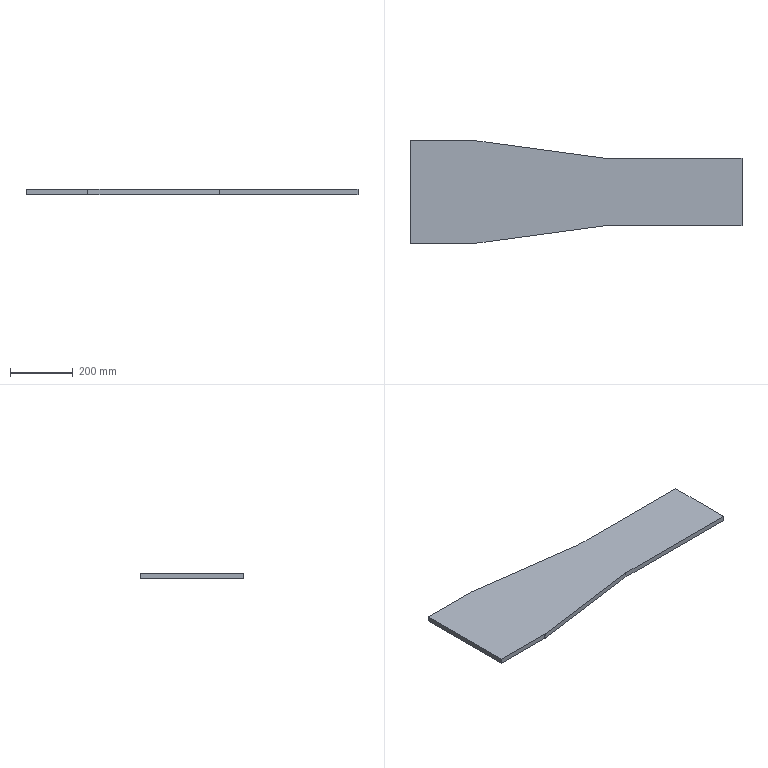Part | SolidWorks | features Extrusion 1 | 1 solid | 12 faces | box 1056 x 330 x 16 mm | volume 4392263 mm3 | plane 10 | cylinder 2 | commonest cylinder face diameters 32 x2
STEP:
#1=CARTESIAN_POINT('',(1056.5,108.,0.));
#2=VERTEX_POINT('',#1);
#3=CARTESIAN_POINT('',(616.5,108.,0.));
#4=VERTEX_POINT('',#3);
#5=CARTESIAN_POINT('',(1056.5,108.,0.));
#6=DIRECTION('',(-1.,0.,0.));
#7=VECTOR('',#6,1000.);
#8=LINE('',#5,#7);
#9=EDGE_CURVE('',#2,#4,#8,.T.);
#10=ORIENTED_EDGE('',*,*,#9,.T.);
#11=CARTESIAN_POINT('',(616.5,108.,16.));
#12=VERTEX_POINT('',#11);
#13=CARTESIAN_POINT('',(616.5,108.,16.));
#14=DIRECTION('',(0.,0.,-1.));
#15=VECTOR('',#14,1000.);
#16=LINE('',#13,#15);
#17=EDGE_CURVE('',#12,#4,#16,.T.);
#18=ORIENTED_EDGE('',*,*,#17,.F.);
#19=CARTESIAN_POINT('',(1056.5,108.,16.));
#20=VERTEX_POINT('',#19);
#21=CARTESIAN_POINT('',(1056.5,108.,16.));
#22=DIRECTION('',(-1.,0.,0.));
#23=VECTOR('',#22,1000.);
#24=LINE('',#21,#23);
#25=EDGE_CURVE('',#20,#12,#24,.T.);
#26=ORIENTED_EDGE('',*,*,#25,.F.);
#27=CARTESIAN_POINT('',(1056.5,108.,16.));
#28=DIRECTION('',(0.,0.,-1.));
#29=VECTOR('',#28,1000.);
#30=LINE('',#27,#29);
#31=EDGE_CURVE('',#20,#2,#30,.T.);
#32=ORIENTED_EDGE('',*,*,#31,.T.);
#33=EDGE_LOOP('',(#10,#18,#26,#32));
#34=FACE_OUTER_BOUND('',#33,.T.);
#35=CARTESIAN_POINT('',(1056.5,108.,16.));
#36=DIRECTION('',(0.,-1.,0.));
#37=DIRECTION('',(1.,0.,0.));
#38=AXIS2_PLACEMENT_3D('',#35,#36,#37);
#39=PLANE('',#38);
#40=ADVANCED_FACE('',(#34),#39,.F.);
#41=CARTESIAN_POINT('',(197.07,164.855,0.));
#42=VERTEX_POINT('',#41);
#43=CARTESIAN_POINT('',(616.5,108.,0.));
#44=DIRECTION('',(-0.9909,0.1343,0.));
#45=VECTOR('',#44,1000.);
#46=LINE('',#43,#45);
#47=EDGE_CURVE('',#4,#42,#46,.T.);
#48=ORIENTED_EDGE('',*,*,#47,.T.);
#49=CARTESIAN_POINT('',(197.07,164.855,16.));
#50=VERTEX_POINT('',#49);
#51=CARTESIAN_POINT('',(197.07,164.855,16.));
#52=DIRECTION('',(0.,0.,-1.));
#53=VECTOR('',#52,1000.);
#54=LINE('',#51,#53);
#55=EDGE_CURVE('',#50,#42,#54,.T.);
#56=ORIENTED_EDGE('',*,*,#55,.F.);
#57=CARTESIAN_POINT('',(616.5,108.,16.));
#58=DIRECTION('',(-0.9909,0.1343,0.));
#59=VECTOR('',#58,1000.);
#60=LINE('',#57,#59);
#61=EDGE_CURVE('',#12,#50,#60,.T.);
#62=ORIENTED_EDGE('',*,*,#61,.F.);
#63=ORIENTED_EDGE('',*,*,#17,.T.);
#64=EDGE_LOOP('',(#48,#56,#62,#63));
#65=FACE_OUTER_BOUND('',#64,.T.);
#66=CARTESIAN_POINT('',(616.5,108.,16.));
#67=DIRECTION('',(-0.1343,-0.9909,0.));
#68=DIRECTION('',(0.9909,-0.1343,0.));
#69=AXIS2_PLACEMENT_3D('',#66,#67,#68);
#70=PLANE('',#69);
#71=ADVANCED_FACE('',(#65),#70,.F.);
#72=CARTESIAN_POINT('',(194.921,165.,0.));
#73=VERTEX_POINT('',#72);
#74=CARTESIAN_POINT('',(194.921,149.,0.));
#75=DIRECTION('',(0.,0.,1.));
#76=DIRECTION('',(-1.,0.,0.));
#77=AXIS2_PLACEMENT_3D('',#74,#75,#76);
#78=CIRCLE('',#77,16.);
#79=EDGE_CURVE('',#42,#73,#78,.T.);
#80=ORIENTED_EDGE('',*,*,#79,.T.);
#81=CARTESIAN_POINT('',(194.921,165.,16.));
#82=VERTEX_POINT('',#81);
#83=CARTESIAN_POINT('',(194.921,165.,16.));
#84=DIRECTION('',(0.,0.,-1.));
#85=VECTOR('',#84,1000.);
#86=LINE('',#83,#85);
#87=EDGE_CURVE('',#82,#73,#86,.T.);
#88=ORIENTED_EDGE('',*,*,#87,.F.);
#89=CARTESIAN_POINT('',(194.921,149.,16.));
#90=DIRECTION('',(0.,0.,1.));
#91=DIRECTION('',(-1.,0.,0.));
#92=AXIS2_PLACEMENT_3D('',#89,#90,#91);
#93=CIRCLE('',#92,16.);
#94=EDGE_CURVE('',#50,#82,#93,.T.);
#95=ORIENTED_EDGE('',*,*,#94,.F.);
#96=ORIENTED_EDGE('',*,*,#55,.T.);
#97=EDGE_LOOP('',(#80,#88,#95,#96));
#98=FACE_OUTER_BOUND('',#97,.T.);
#99=CARTESIAN_POINT('',(194.921,149.,16.));
#100=DIRECTION('',(0.,0.,-1.));
#101=DIRECTION('',(-1.,0.,0.));
#102=AXIS2_PLACEMENT_3D('',#99,#100,#101);
#103=CYLINDRICAL_SURFACE('',#102,16.);
#104=ADVANCED_FACE('',(#98),#103,.T.);
#105=CARTESIAN_POINT('',(0.,165.,0.));
#106=VERTEX_POINT('',#105);
#107=CARTESIAN_POINT('',(0.,165.,0.));
#108=DIRECTION('',(-1.,0.,0.));
#109=VECTOR('',#108,1000.);
#110=LINE('',#107,#109);
#111=EDGE_CURVE('',#73,#106,#110,.T.);
#112=ORIENTED_EDGE('',*,*,#111,.T.);
#113=CARTESIAN_POINT('',(0.,165.,16.));
#114=VERTEX_POINT('',#113);
#115=CARTESIAN_POINT('',(0.,165.,16.));
#116=DIRECTION('',(0.,0.,-1.));
#117=VECTOR('',#116,1000.);
#118=LINE('',#115,#117);
#119=EDGE_CURVE('',#114,#106,#118,.T.);
#120=ORIENTED_EDGE('',*,*,#119,.F.);
#121=CARTESIAN_POINT('',(0.,165.,16.));
#122=DIRECTION('',(-1.,0.,0.));
#123=VECTOR('',#122,1000.);
#124=LINE('',#121,#123);
#125=EDGE_CURVE('',#82,#114,#124,.T.);
#126=ORIENTED_EDGE('',*,*,#125,.F.);
#127=ORIENTED_EDGE('',*,*,#87,.T.);
#128=EDGE_LOOP('',(#112,#120,#126,#127));
#129=FACE_OUTER_BOUND('',#128,.T.);
#130=CARTESIAN_POINT('',(0.,165.,16.));
#131=DIRECTION('',(0.,-1.,0.));
#132=DIRECTION('',(0.,0.,-1.));
#133=AXIS2_PLACEMENT_3D('',#130,#131,#132);
#134=PLANE('',#133);
#135=ADVANCED_FACE('',(#129),#134,.F.);
#136=CARTESIAN_POINT('',(0.,-165.,0.));
#137=VERTEX_POINT('',#136);
#138=CARTESIAN_POINT('',(0.,-165.,0.));
#139=DIRECTION('',(0.,-1.,0.));
#140=VECTOR('',#139,1000.);
#141=LINE('',#138,#140);
#142=EDGE_CURVE('',#106,#137,#141,.T.);
#143=ORIENTED_EDGE('',*,*,#142,.T.);
#144=CARTESIAN_POINT('',(0.,-165.,16.));
#145=VERTEX_POINT('',#144);
#146=CARTESIAN_POINT('',(0.,-165.,16.));
#147=DIRECTION('',(0.,0.,-1.));
#148=VECTOR('',#147,1000.);
#149=LINE('',#146,#148);
#150=EDGE_CURVE('',#145,#137,#149,.T.);
#151=ORIENTED_EDGE('',*,*,#150,.F.);
#152=CARTESIAN_POINT('',(0.,-165.,16.));
#153=DIRECTION('',(0.,-1.,0.));
#154=VECTOR('',#153,1000.);
#155=LINE('',#152,#154);
#156=EDGE_CURVE('',#114,#145,#155,.T.);
#157=ORIENTED_EDGE('',*,*,#156,.F.);
#158=ORIENTED_EDGE('',*,*,#119,.T.);
#159=EDGE_LOOP('',(#143,#151,#157,#158));
#160=FACE_OUTER_BOUND('',#159,.T.);
#161=CARTESIAN_POINT('',(0.,-165.,16.));
#162=DIRECTION('',(1.,0.,0.));
#163=DIRECTION('',(0.,0.,-1.));
#164=AXIS2_PLACEMENT_3D('',#161,#162,#163);
#165=PLANE('',#164);
#166=ADVANCED_FACE('',(#160),#165,.F.);
#167=CARTESIAN_POINT('',(194.921,-165.,0.));
#168=VERTEX_POINT('',#167);
#169=CARTESIAN_POINT('',(0.,-165.,0.));
#170=DIRECTION('',(1.,0.,0.));
#171=VECTOR('',#170,1000.);
#172=LINE('',#169,#171);
#173=EDGE_CURVE('',#137,#168,#172,.T.);
#174=ORIENTED_EDGE('',*,*,#173,.T.);
#175=CARTESIAN_POINT('',(194.921,-165.,16.));
#176=VERTEX_POINT('',#175);
#177=CARTESIAN_POINT('',(194.921,-165.,16.));
#178=DIRECTION('',(0.,0.,-1.));
#179=VECTOR('',#178,1000.);
#180=LINE('',#177,#179);
#181=EDGE_CURVE('',#176,#168,#180,.T.);
#182=ORIENTED_EDGE('',*,*,#181,.F.);
#183=CARTESIAN_POINT('',(0.,-165.,16.));
#184=DIRECTION('',(1.,0.,0.));
#185=VECTOR('',#184,1000.);
#186=LINE('',#183,#185);
#187=EDGE_CURVE('',#145,#176,#186,.T.);
#188=ORIENTED_EDGE('',*,*,#187,.F.);
#189=ORIENTED_EDGE('',*,*,#150,.T.);
#190=EDGE_LOOP('',(#174,#182,#188,#189));
#191=FACE_OUTER_BOUND('',#190,.T.);
#192=CARTESIAN_POINT('',(0.,-165.,16.));
#193=DIRECTION('',(0.,1.,0.));
#194=DIRECTION('',(0.,0.,1.));
#195=AXIS2_PLACEMENT_3D('',#192,#193,#194);
#196=PLANE('',#195);
#197=ADVANCED_FACE('',(#191),#196,.F.);
#198=CARTESIAN_POINT('',(197.07,-164.855,0.));
#199=VERTEX_POINT('',#198);
#200=CARTESIAN_POINT('',(194.921,-149.,0.));
#201=DIRECTION('',(0.,0.,1.));
#202=DIRECTION('',(1.,0.,0.));
#203=AXIS2_PLACEMENT_3D('',#200,#201,#202);
#204=CIRCLE('',#203,16.);
#205=EDGE_CURVE('',#168,#199,#204,.T.);
#206=ORIENTED_EDGE('',*,*,#205,.T.);
#207=CARTESIAN_POINT('',(197.07,-164.855,16.));
#208=VERTEX_POINT('',#207);
#209=CARTESIAN_POINT('',(197.07,-164.855,16.));
#210=DIRECTION('',(0.,0.,-1.));
#211=VECTOR('',#210,1000.);
#212=LINE('',#209,#211);
#213=EDGE_CURVE('',#208,#199,#212,.T.);
#214=ORIENTED_EDGE('',*,*,#213,.F.);
#215=CARTESIAN_POINT('',(194.921,-149.,16.));
#216=DIRECTION('',(0.,0.,1.));
#217=DIRECTION('',(1.,0.,0.));
#218=AXIS2_PLACEMENT_3D('',#215,#216,#217);
#219=CIRCLE('',#218,16.);
#220=EDGE_CURVE('',#176,#208,#219,.T.);
#221=ORIENTED_EDGE('',*,*,#220,.F.);
#222=ORIENTED_EDGE('',*,*,#181,.T.);
#223=EDGE_LOOP('',(#206,#214,#221,#222));
#224=FACE_OUTER_BOUND('',#223,.T.);
#225=CARTESIAN_POINT('',(194.921,-149.,16.));
#226=DIRECTION('',(0.,0.,-1.));
#227=DIRECTION('',(-1.,0.,0.));
#228=AXIS2_PLACEMENT_3D('',#225,#226,#227);
#229=CYLINDRICAL_SURFACE('',#228,16.);
#230=ADVANCED_FACE('',(#224),#229,.T.);
#231=CARTESIAN_POINT('',(616.5,-108.,0.));
#232=VERTEX_POINT('',#231);
#233=CARTESIAN_POINT('',(616.5,-108.,0.));
#234=DIRECTION('',(0.9909,0.1343,0.));
#235=VECTOR('',#234,1000.);
#236=LINE('',#233,#235);
#237=EDGE_CURVE('',#199,#232,#236,.T.);
#238=ORIENTED_EDGE('',*,*,#237,.T.);
#239=CARTESIAN_POINT('',(616.5,-108.,16.));
#240=VERTEX_POINT('',#239);
#241=CARTESIAN_POINT('',(616.5,-108.,16.));
#242=DIRECTION('',(0.,0.,-1.));
#243=VECTOR('',#242,1000.);
#244=LINE('',#241,#243);
#245=EDGE_CURVE('',#240,#232,#244,.T.);
#246=ORIENTED_EDGE('',*,*,#245,.F.);
#247=CARTESIAN_POINT('',(616.5,-108.,16.));
#248=DIRECTION('',(0.9909,0.1343,0.));
#249=VECTOR('',#248,1000.);
#250=LINE('',#247,#249);
#251=EDGE_CURVE('',#208,#240,#250,.T.);
#252=ORIENTED_EDGE('',*,*,#251,.F.);
#253=ORIENTED_EDGE('',*,*,#213,.T.);
#254=EDGE_LOOP('',(#238,#246,#252,#253));
#255=FACE_OUTER_BOUND('',#254,.T.);
#256=CARTESIAN_POINT('',(616.5,-108.,16.));
#257=DIRECTION('',(-0.1343,0.9909,0.));
#258=DIRECTION('',(-0.9909,-0.1343,0.));
#259=AXIS2_PLACEMENT_3D('',#256,#257,#258);
#260=PLANE('',#259);
#261=ADVANCED_FACE('',(#255),#260,.F.);
#262=CARTESIAN_POINT('',(1056.5,-108.,0.));
#263=VERTEX_POINT('',#262);
#264=CARTESIAN_POINT('',(1056.5,-108.,0.));
#265=DIRECTION('',(1.,0.,0.));
#266=VECTOR('',#265,1000.);
#267=LINE('',#264,#266);
#268=EDGE_CURVE('',#232,#263,#267,.T.);
#269=ORIENTED_EDGE('',*,*,#268,.T.);
#270=CARTESIAN_POINT('',(1056.5,-108.,16.));
#271=VERTEX_POINT('',#270);
#272=CARTESIAN_POINT('',(1056.5,-108.,16.));
#273=DIRECTION('',(0.,0.,-1.));
#274=VECTOR('',#273,1000.);
#275=LINE('',#272,#274);
#276=EDGE_CURVE('',#271,#263,#275,.T.);
#277=ORIENTED_EDGE('',*,*,#276,.F.);
#278=CARTESIAN_POINT('',(1056.5,-108.,16.));
#279=DIRECTION('',(1.,0.,0.));
#280=VECTOR('',#279,1000.);
#281=LINE('',#278,#280);
#282=EDGE_CURVE('',#240,#271,#281,.T.);
#283=ORIENTED_EDGE('',*,*,#282,.F.);
#284=ORIENTED_EDGE('',*,*,#245,.T.);
#285=EDGE_LOOP('',(#269,#277,#283,#284));
#286=FACE_OUTER_BOUND('',#285,.T.);
#287=CARTESIAN_POINT('',(1056.5,-108.,16.));
#288=DIRECTION('',(0.,1.,0.));
#289=DIRECTION('',(-1.,0.,0.));
#290=AXIS2_PLACEMENT_3D('',#287,#288,#289);
#291=PLANE('',#290);
#292=ADVANCED_FACE('',(#286),#291,.F.);
#293=CARTESIAN_POINT('',(1056.5,108.,0.));
#294=DIRECTION('',(0.,1.,0.));
#295=VECTOR('',#294,1000.);
#296=LINE('',#293,#295);
#297=EDGE_CURVE('',#263,#2,#296,.T.);
#298=ORIENTED_EDGE('',*,*,#297,.T.);
#299=ORIENTED_EDGE('',*,*,#31,.F.);
#300=CARTESIAN_POINT('',(1056.5,108.,16.));
#301=DIRECTION('',(0.,1.,0.));
#302=VECTOR('',#301,1000.);
#303=LINE('',#300,#302);
#304=EDGE_CURVE('',#271,#20,#303,.T.);
#305=ORIENTED_EDGE('',*,*,#304,.F.);
#306=ORIENTED_EDGE('',*,*,#276,.T.);
#307=EDGE_LOOP('',(#298,#299,#305,#306));
#308=FACE_OUTER_BOUND('',#307,.T.);
#309=CARTESIAN_POINT('',(1056.5,108.,16.));
#310=DIRECTION('',(-1.,0.,0.));
#311=DIRECTION('',(0.,0.,1.));
#312=AXIS2_PLACEMENT_3D('',#309,#310,#311);
#313=PLANE('',#312);
#314=ADVANCED_FACE('',(#308),#313,.F.);
#315=ORIENTED_EDGE('',*,*,#25,.T.);
#316=ORIENTED_EDGE('',*,*,#61,.T.);
#317=ORIENTED_EDGE('',*,*,#94,.T.);
#318=ORIENTED_EDGE('',*,*,#125,.T.);
#319=ORIENTED_EDGE('',*,*,#156,.T.);
#320=ORIENTED_EDGE('',*,*,#187,.T.);
#321=ORIENTED_EDGE('',*,*,#220,.T.);
#322=ORIENTED_EDGE('',*,*,#251,.T.);
#323=ORIENTED_EDGE('',*,*,#282,.T.);
#324=ORIENTED_EDGE('',*,*,#304,.T.);
#325=EDGE_LOOP('',(#315,#316,#317,#318,#319,#320,#321,#322,#323,#324));
#326=FACE_OUTER_BOUND('',#325,.T.);
#327=CARTESIAN_POINT('',(194.921,149.,16.));
#328=DIRECTION('',(0.,0.,-1.));
#329=DIRECTION('',(-1.,0.,0.));
#330=AXIS2_PLACEMENT_3D('',#327,#328,#329);
#331=PLANE('',#330);
#332=ADVANCED_FACE('',(#326),#331,.F.);
#333=ORIENTED_EDGE('',*,*,#9,.F.);
#334=ORIENTED_EDGE('',*,*,#297,.F.);
#335=ORIENTED_EDGE('',*,*,#268,.F.);
#336=ORIENTED_EDGE('',*,*,#237,.F.);
#337=ORIENTED_EDGE('',*,*,#205,.F.);
#338=ORIENTED_EDGE('',*,*,#173,.F.);
#339=ORIENTED_EDGE('',*,*,#142,.F.);
#340=ORIENTED_EDGE('',*,*,#111,.F.);
#341=ORIENTED_EDGE('',*,*,#79,.F.);
#342=ORIENTED_EDGE('',*,*,#47,.F.);
#343=EDGE_LOOP('',(#333,#334,#335,#336,#337,#338,#339,#340,#341,#342));
#344=FACE_OUTER_BOUND('',#343,.T.);
#345=CARTESIAN_POINT('',(194.921,149.,0.));
#346=DIRECTION('',(0.,0.,-1.));
#347=DIRECTION('',(-1.,0.,0.));
#348=AXIS2_PLACEMENT_3D('',#345,#346,#347);
#349=PLANE('',#348);
#350=ADVANCED_FACE('',(#344),#349,.T.);
#351=CLOSED_SHELL('',(#40,#71,#104,#135,#166,#197,#230,#261,#292,#314,#332,#350));
#352=MANIFOLD_SOLID_BREP('',#351);
#353=CARTESIAN_POINT('',(0.,0.,0.));
#354=DIRECTION('',(0.,0.,1.));
#355=DIRECTION('',(1.,0.,0.));
#356=AXIS2_PLACEMENT_3D('',#353,#354,#355);
#357=(LENGTH_UNIT()NAMED_UNIT(*)SI_UNIT(.MILLI.,.METRE.));
#358=UNCERTAINTY_MEASURE_WITH_UNIT(LENGTH_MEASURE(0.00001),#357,'','');
#359=(NAMED_UNIT(*)PLANE_ANGLE_UNIT()SI_UNIT($,.RADIAN.));
#360=(NAMED_UNIT(*)SI_UNIT($,.STERADIAN.)SOLID_ANGLE_UNIT());
#361=(GEOMETRIC_REPRESENTATION_CONTEXT(3)GLOBAL_UNCERTAINTY_ASSIGNED_CONTEXT((#358))GLOBAL_UNIT_ASSIGNED_CONTEXT((#357,#359,#360))REPRESENTATION_CONTEXT('',''));
#362=ADVANCED_BREP_SHAPE_REPRESENTATION('',(#352,#356),#361);